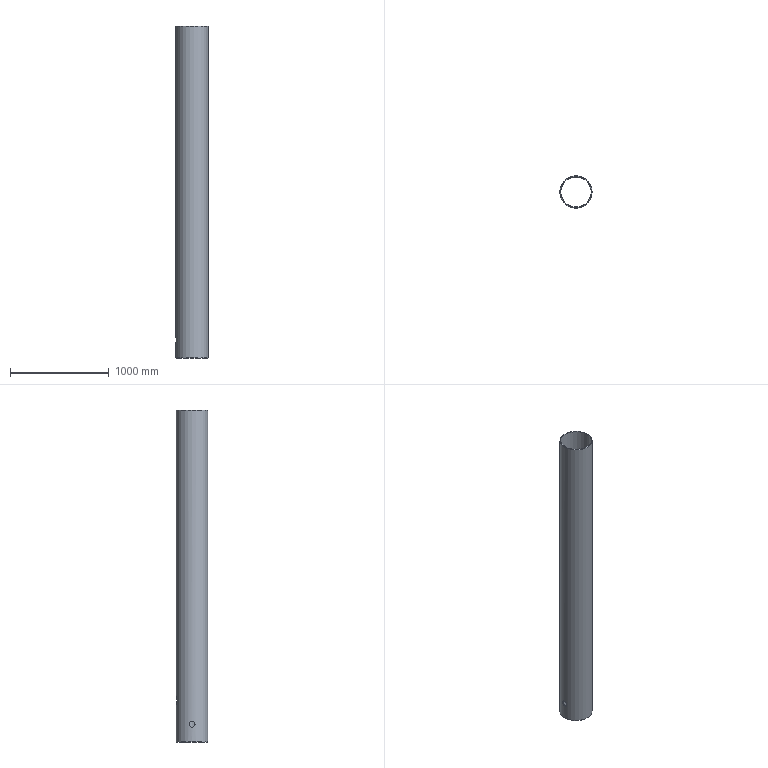Part | NX | features DATUM_CSYS 3, EXTRUDE 2, SKETCH 2, CHAMFER 1, CYLINDER 1, SHELL 1 | 1 solid | 8 faces | box 325 x 325 x 3360 mm | volume 26652772 mm3 | cylinder 4 | plane 2 | cone 2 | commonest cylinder face diameters 60 x1 114 x1 309 x1 325 x1
STEP:
#1=CARTESIAN_POINT('',(-162.5,0.,150.));
#2=VERTEX_POINT('',#1);
#3=CARTESIAN_POINT('',(-162.196,11.848,151.588));
#4=CARTESIAN_POINT('',(-162.651,-0.009709,149.209));
#5=CARTESIAN_POINT('',(-162.198,-11.809,151.576));
#6=CARTESIAN_POINT('',(-161.11,-21.766,158.243));
#7=CARTESIAN_POINT('',(-160.015,-28.424,168.193));
#8=CARTESIAN_POINT('',(-159.553,-30.784,179.98));
#9=CARTESIAN_POINT('',(-160.012,-28.438,191.782));
#10=CARTESIAN_POINT('',(-161.11,-21.767,201.759));
#11=CARTESIAN_POINT('',(-162.199,-11.805,208.427));
#12=CARTESIAN_POINT('',(-162.65,-0.01225,210.784));
#13=CARTESIAN_POINT('',(-162.2,11.782,208.436));
#14=CARTESIAN_POINT('',(-161.114,21.742,201.781));
#15=CARTESIAN_POINT('',(-160.016,28.416,191.833));
#16=CARTESIAN_POINT('',(-159.553,30.787,180.022));
#17=CARTESIAN_POINT('',(-160.013,28.436,168.213));
#18=CARTESIAN_POINT('',(-161.109,21.773,158.254));
#19=CARTESIAN_POINT('',(-162.196,11.848,151.588));
#20=CARTESIAN_POINT('',(-162.651,-0.009709,149.209));
#21=CARTESIAN_POINT('',(-162.198,-11.809,151.576));
#22=B_SPLINE_CURVE_WITH_KNOTS('',3,(#3,#4,#5,#6,#7,#8,#9,#10,#11,#12,#13,#14,#15,#16,#17,#18,#19,#20,#21),.UNSPECIFIED.,.T.,.F.,(1,1,1,1,1,1,1,1,1,1,1,1,1,1,1,1,1,1,1,1,1,1,1),(-0.03524,-0.0235,-0.01175,0.,0.01175,0.0235,0.03524,0.04699,0.05874,0.07049,0.08224,0.09398,0.1057,0.1175,0.1292,0.141,0.1527,0.1645,0.1762,0.188,0.1997,0.2115,0.2232),.UNSPECIFIED.);
#23=EDGE_CURVE('',#2,#2,#22,.T.);
#24=ORIENTED_EDGE('',*,*,#23,.F.);
#25=EDGE_LOOP('',(#24));
#26=FACE_BOUND('',#25,.T.);
#27=CARTESIAN_POINT('',(162.5,0.,3357.5));
#28=VERTEX_POINT('',#27);
#29=CARTESIAN_POINT('',(0.,0.,3357.5));
#30=DIRECTION('',(0.,0.,1.));
#31=DIRECTION('',(1.,0.,0.));
#32=AXIS2_PLACEMENT_3D('',#29,#30,#31);
#33=CIRCLE('',#32,162.5);
#34=EDGE_CURVE('',#28,#28,#33,.F.);
#35=ORIENTED_EDGE('',*,*,#34,.T.);
#36=EDGE_LOOP('',(#35));
#37=FACE_BOUND('',#36,.T.);
#38=CARTESIAN_POINT('',(-162.5,0.,2.5));
#39=VERTEX_POINT('',#38);
#40=CARTESIAN_POINT('',(0.,0.,2.5));
#41=DIRECTION('',(0.,0.,-1.));
#42=DIRECTION('',(-1.,0.,0.));
#43=AXIS2_PLACEMENT_3D('',#40,#41,#42);
#44=CIRCLE('',#43,162.5);
#45=EDGE_CURVE('',#39,#39,#44,.F.);
#46=ORIENTED_EDGE('',*,*,#45,.T.);
#47=EDGE_LOOP('',(#46));
#48=FACE_BOUND('',#47,.T.);
#49=CARTESIAN_POINT('',(0.,162.5,363.));
#50=VERTEX_POINT('',#49);
#51=CARTESIAN_POINT('',(-5.67,162.434,363.189));
#52=CARTESIAN_POINT('',(1.9,162.566,362.813));
#53=CARTESIAN_POINT('',(11.251,162.238,363.741));
#54=CARTESIAN_POINT('',(22.111,161.103,367.065));
#55=CARTESIAN_POINT('',(31.923,159.427,372.341));
#56=CARTESIAN_POINT('',(40.588,157.42,379.464));
#57=CARTESIAN_POINT('',(47.651,155.401,388.066));
#58=CARTESIAN_POINT('',(52.068,153.944,396.293));
#59=CARTESIAN_POINT('',(54.59,153.059,403.281));
#60=CARTESIAN_POINT('',(56.447,152.385,410.637));
#61=CARTESIAN_POINT('',(57.372,152.034,419.919));
#62=CARTESIAN_POINT('',(56.25,152.459,431.302));
#63=CARTESIAN_POINT('',(53.52,153.448,440.229));
#64=CARTESIAN_POINT('',(50.293,154.53,447.019));
#65=CARTESIAN_POINT('',(46.489,155.733,453.343));
#66=CARTESIAN_POINT('',(40.532,157.433,460.588));
#67=CARTESIAN_POINT('',(31.994,159.414,467.612));
#68=CARTESIAN_POINT('',(22.033,161.113,472.966));
#69=CARTESIAN_POINT('',(13.147,162.042,475.687));
#70=CARTESIAN_POINT('',(5.628,162.435,476.816));
#71=CARTESIAN_POINT('',(0.02166,162.532,477.091));
#72=CARTESIAN_POINT('',(-5.585,162.437,476.82));
#73=CARTESIAN_POINT('',(-13.103,162.046,475.698));
#74=CARTESIAN_POINT('',(-22.02,161.115,472.973));
#75=CARTESIAN_POINT('',(-31.981,159.416,467.622));
#76=CARTESIAN_POINT('',(-39.111,157.763,461.756));
#77=CARTESIAN_POINT('',(-44.132,156.407,456.219));
#78=CARTESIAN_POINT('',(-47.426,155.436,451.779));
#79=CARTESIAN_POINT('',(-50.287,154.532,447.032));
#80=CARTESIAN_POINT('',(-53.52,153.448,440.227));
#81=CARTESIAN_POINT('',(-56.238,152.463,431.347));
#82=CARTESIAN_POINT('',(-57.374,152.033,419.959));
#83=CARTESIAN_POINT('',(-56.45,152.384,410.659));
#84=CARTESIAN_POINT('',(-54.598,153.057,403.304));
#85=CARTESIAN_POINT('',(-52.7,153.723,398.047));
#86=CARTESIAN_POINT('',(-50.314,154.523,393.017));
#87=CARTESIAN_POINT('',(-46.44,155.748,386.584));
#88=CARTESIAN_POINT('',(-40.59,157.42,379.468));
#89=CARTESIAN_POINT('',(-31.887,159.434,372.317));
#90=CARTESIAN_POINT('',(-23.755,160.822,367.949));
#91=CARTESIAN_POINT('',(-16.637,161.677,365.384));
#92=CARTESIAN_POINT('',(-11.201,162.144,364.019));
#93=CARTESIAN_POINT('',(-5.67,162.434,363.189));
#94=CARTESIAN_POINT('',(1.9,162.566,362.813));
#95=CARTESIAN_POINT('',(11.251,162.238,363.741));
#96=B_SPLINE_CURVE_WITH_KNOTS('',3,(#51,#52,#53,#54,#55,#56,#57,#58,#59,#60,#61,#62,#63,#64,#65,#66,#67,#68,#69,#70,#71,#72,#73,#74,#75,#76,#77,#78,#79,#80,#81,#82,#83,#84,#85,#86,#87,#88,#89,#90,#91,#92,#93,#94,#95),.UNSPECIFIED.,.T.,.F.,(1,1,1,1,1,1,1,1,1,1,1,1,1,1,1,1,1,1,1,1,1,1,1,1,1,1,1,1,1,1,1,1,1,1,1,1,1,1,1,1,1,1,1,1,1,1,1,1,1),(-0.01684,-0.01123,-0.005613,0.,0.01123,0.02245,0.03368,0.04491,0.05613,0.06736,0.07297,0.07859,0.08981,0.101,0.1123,0.1179,0.1235,0.1347,0.1459,0.1572,0.1684,0.174,0.1796,0.1852,0.1909,0.2021,0.2133,0.2245,0.2301,0.2358,0.2414,0.247,0.2582,0.2694,0.2807,0.2863,0.2919,0.2975,0.3031,0.3143,0.3256,0.3368,0.3424,0.348,0.3536,0.3593,0.3705,0.3817,0.3929),.UNSPECIFIED.);
#97=EDGE_CURVE('',#50,#50,#96,.T.);
#98=ORIENTED_EDGE('',*,*,#97,.T.);
#99=EDGE_LOOP('',(#98));
#100=FACE_BOUND('',#99,.T.);
#101=CARTESIAN_POINT('',(0.,0.,0.));
#102=DIRECTION('',(0.,0.,1.));
#103=DIRECTION('',(1.,0.,0.));
#104=AXIS2_PLACEMENT_3D('',#101,#102,#103);
#105=CYLINDRICAL_SURFACE('',#104,162.5);
#106=ADVANCED_FACE('',(#26,#37,#48,#100),#105,.T.);
#107=CARTESIAN_POINT('',(-154.5,0.,150.));
#108=VERTEX_POINT('',#107);
#109=CARTESIAN_POINT('',(-154.18,11.85,151.589));
#110=CARTESIAN_POINT('',(-154.659,-0.009625,149.209));
#111=CARTESIAN_POINT('',(-154.182,-11.812,151.577));
#112=CARTESIAN_POINT('',(-153.038,-21.766,158.243));
#113=CARTESIAN_POINT('',(-151.884,-28.423,168.19));
#114=CARTESIAN_POINT('',(-151.398,-30.785,179.98));
#115=CARTESIAN_POINT('',(-151.881,-28.437,191.784));
#116=CARTESIAN_POINT('',(-153.038,-21.766,201.76));
#117=CARTESIAN_POINT('',(-154.183,-11.807,208.426));
#118=CARTESIAN_POINT('',(-154.658,-0.01248,210.785));
#119=CARTESIAN_POINT('',(-154.185,11.784,208.435));
#120=CARTESIAN_POINT('',(-153.041,21.742,201.78));
#121=CARTESIAN_POINT('',(-151.886,28.415,191.835));
#122=CARTESIAN_POINT('',(-151.397,30.788,180.021));
#123=CARTESIAN_POINT('',(-151.882,28.435,168.21));
#124=CARTESIAN_POINT('',(-153.036,21.772,158.254));
#125=CARTESIAN_POINT('',(-154.18,11.85,151.589));
#126=CARTESIAN_POINT('',(-154.659,-0.009625,149.209));
#127=CARTESIAN_POINT('',(-154.182,-11.812,151.577));
#128=B_SPLINE_CURVE_WITH_KNOTS('',3,(#109,#110,#111,#112,#113,#114,#115,#116,#117,#118,#119,#120,#121,#122,#123,#124,#125,#126,#127),.UNSPECIFIED.,.T.,.F.,(1,1,1,1,1,1,1,1,1,1,1,1,1,1,1,1,1,1,1,1,1,1,1),(-0.03525,-0.0235,-0.01175,0.,0.01175,0.0235,0.03525,0.047,0.05875,0.0705,0.08225,0.09401,0.1058,0.1175,0.1293,0.141,0.1528,0.1645,0.1763,0.188,0.1998,0.2115,0.2233),.UNSPECIFIED.);
#129=EDGE_CURVE('',#108,#108,#128,.T.);
#130=ORIENTED_EDGE('',*,*,#129,.T.);
#131=EDGE_LOOP('',(#130));
#132=FACE_BOUND('',#131,.T.);
#133=CARTESIAN_POINT('',(154.5,0.,3360.));
#134=VERTEX_POINT('',#133);
#135=CARTESIAN_POINT('',(0.,0.,3360.));
#136=DIRECTION('',(0.,0.,1.));
#137=DIRECTION('',(1.,0.,0.));
#138=AXIS2_PLACEMENT_3D('',#135,#136,#137);
#139=CIRCLE('',#138,154.5);
#140=EDGE_CURVE('',#134,#134,#139,.F.);
#141=ORIENTED_EDGE('',*,*,#140,.F.);
#142=EDGE_LOOP('',(#141));
#143=FACE_BOUND('',#142,.T.);
#144=CARTESIAN_POINT('',(-154.5,0.,0.));
#145=VERTEX_POINT('',#144);
#146=CARTESIAN_POINT('',(0.,0.,0.));
#147=DIRECTION('',(0.,0.,-1.));
#148=DIRECTION('',(-1.,0.,0.));
#149=AXIS2_PLACEMENT_3D('',#146,#147,#148);
#150=CIRCLE('',#149,154.5);
#151=EDGE_CURVE('',#145,#145,#150,.F.);
#152=ORIENTED_EDGE('',*,*,#151,.F.);
#153=EDGE_LOOP('',(#152));
#154=FACE_BOUND('',#153,.T.);
#155=CARTESIAN_POINT('',(0.,154.5,363.));
#156=VERTEX_POINT('',#155);
#157=CARTESIAN_POINT('',(-5.673,154.43,363.19));
#158=CARTESIAN_POINT('',(-0.0003286,154.535,362.905));
#159=CARTESIAN_POINT('',(5.674,154.43,363.19));
#160=CARTESIAN_POINT('',(13.055,154.025,364.294));
#161=CARTESIAN_POINT('',(22.131,153.028,367.071));
#162=CARTESIAN_POINT('',(31.933,151.262,372.35));
#163=CARTESIAN_POINT('',(40.589,149.148,379.466));
#164=CARTESIAN_POINT('',(47.65,147.016,388.065));
#165=CARTESIAN_POINT('',(52.062,145.477,396.281));
#166=CARTESIAN_POINT('',(54.587,144.539,403.271));
#167=CARTESIAN_POINT('',(56.446,143.824,410.63));
#168=CARTESIAN_POINT('',(57.372,143.452,419.92));
#169=CARTESIAN_POINT('',(56.253,143.901,431.303));
#170=CARTESIAN_POINT('',(52.952,145.166,442.06));
#171=CARTESIAN_POINT('',(47.661,147.014,451.928));
#172=CARTESIAN_POINT('',(40.535,149.161,460.582));
#173=CARTESIAN_POINT('',(31.998,151.25,467.61));
#174=CARTESIAN_POINT('',(22.047,153.038,472.961));
#175=CARTESIAN_POINT('',(13.152,154.018,475.687));
#176=CARTESIAN_POINT('',(5.628,154.432,476.816));
#177=CARTESIAN_POINT('',(0.0208,154.534,477.091));
#178=CARTESIAN_POINT('',(-5.595,154.433,476.82));
#179=CARTESIAN_POINT('',(-13.121,154.021,475.694));
#180=CARTESIAN_POINT('',(-22.04,153.04,472.965));
#181=CARTESIAN_POINT('',(-31.993,151.251,467.615));
#182=CARTESIAN_POINT('',(-39.126,149.506,461.741));
#183=CARTESIAN_POINT('',(-44.134,148.078,456.215));
#184=CARTESIAN_POINT('',(-47.425,147.053,451.78));
#185=CARTESIAN_POINT('',(-50.288,146.096,447.031));
#186=CARTESIAN_POINT('',(-53.52,144.949,440.226));
#187=CARTESIAN_POINT('',(-56.237,143.907,431.353));
#188=CARTESIAN_POINT('',(-57.375,143.45,419.95));
#189=CARTESIAN_POINT('',(-56.447,143.823,410.638));
#190=CARTESIAN_POINT('',(-54.591,144.538,403.28));
#191=CARTESIAN_POINT('',(-52.693,145.243,398.029));
#192=CARTESIAN_POINT('',(-50.301,146.091,392.994));
#193=CARTESIAN_POINT('',(-46.426,147.387,386.566));
#194=CARTESIAN_POINT('',(-40.58,149.151,379.459));
#195=CARTESIAN_POINT('',(-31.886,151.273,372.317));
#196=CARTESIAN_POINT('',(-23.749,152.735,367.946));
#197=CARTESIAN_POINT('',(-16.628,153.635,365.381));
#198=CARTESIAN_POINT('',(-11.205,154.126,364.02));
#199=CARTESIAN_POINT('',(-5.673,154.43,363.19));
#200=CARTESIAN_POINT('',(-0.0003286,154.535,362.905));
#201=CARTESIAN_POINT('',(5.674,154.43,363.19));
#202=B_SPLINE_CURVE_WITH_KNOTS('',3,(#157,#158,#159,#160,#161,#162,#163,#164,#165,#166,#167,#168,#169,#170,#171,#172,#173,#174,#175,#176,#177,#178,#179,#180,#181,#182,#183,#184,#185,#186,#187,#188,#189,#190,#191,#192,#193,#194,#195,#196,#197,#198,#199,#200,#201),.UNSPECIFIED.,.T.,.F.,(1,1,1,1,1,1,1,1,1,1,1,1,1,1,1,1,1,1,1,1,1,1,1,1,1,1,1,1,1,1,1,1,1,1,1,1,1,1,1,1,1,1,1,1,1,1,1,1,1),(-0.01686,-0.01124,-0.005618,0.,0.005618,0.01124,0.02247,0.03371,0.04495,0.05618,0.06742,0.07304,0.07866,0.0899,0.1011,0.1124,0.1236,0.1348,0.1461,0.1573,0.1686,0.1742,0.1798,0.1854,0.191,0.2023,0.2135,0.2247,0.2304,0.236,0.2416,0.2472,0.2585,0.2697,0.2809,0.2865,0.2922,0.2978,0.3034,0.3146,0.3259,0.3371,0.3427,0.3483,0.354,0.3596,0.3652,0.3708,0.3821),.UNSPECIFIED.);
#203=EDGE_CURVE('',#156,#156,#202,.T.);
#204=ORIENTED_EDGE('',*,*,#203,.F.);
#205=EDGE_LOOP('',(#204));
#206=FACE_BOUND('',#205,.T.);
#207=CARTESIAN_POINT('',(0.,0.,0.));
#208=DIRECTION('',(0.,0.,1.));
#209=DIRECTION('',(1.,0.,0.));
#210=AXIS2_PLACEMENT_3D('',#207,#208,#209);
#211=CYLINDRICAL_SURFACE('',#210,154.5);
#212=ADVANCED_FACE('',(#132,#143,#154,#206),#211,.F.);
#213=CARTESIAN_POINT('',(158.17,0.,3360.));
#214=VERTEX_POINT('',#213);
#215=CARTESIAN_POINT('',(0.,0.,3360.));
#216=DIRECTION('',(0.,0.,1.));
#217=DIRECTION('',(1.,0.,0.));
#218=AXIS2_PLACEMENT_3D('',#215,#216,#217);
#219=CIRCLE('',#218,158.17);
#220=EDGE_CURVE('',#214,#214,#219,.T.);
#221=ORIENTED_EDGE('',*,*,#220,.T.);
#222=EDGE_LOOP('',(#221));
#223=FACE_BOUND('',#222,.T.);
#224=ORIENTED_EDGE('',*,*,#140,.T.);
#225=EDGE_LOOP('',(#224));
#226=FACE_BOUND('',#225,.T.);
#227=CARTESIAN_POINT('',(0.,0.,3360.));
#228=DIRECTION('',(0.,0.,1.));
#229=DIRECTION('',(1.,0.,0.));
#230=AXIS2_PLACEMENT_3D('',#227,#228,#229);
#231=PLANE('',#230);
#232=ADVANCED_FACE('',(#223,#226),#231,.T.);
#233=CARTESIAN_POINT('',(-158.17,0.,0.));
#234=VERTEX_POINT('',#233);
#235=CARTESIAN_POINT('',(0.,0.,0.));
#236=DIRECTION('',(0.,0.,-1.));
#237=DIRECTION('',(-1.,0.,0.));
#238=AXIS2_PLACEMENT_3D('',#235,#236,#237);
#239=CIRCLE('',#238,158.17);
#240=EDGE_CURVE('',#234,#234,#239,.T.);
#241=ORIENTED_EDGE('',*,*,#240,.T.);
#242=EDGE_LOOP('',(#241));
#243=FACE_BOUND('',#242,.T.);
#244=ORIENTED_EDGE('',*,*,#151,.T.);
#245=EDGE_LOOP('',(#244));
#246=FACE_BOUND('',#245,.T.);
#247=CARTESIAN_POINT('',(0.,0.,0.));
#248=DIRECTION('',(0.,0.,-1.));
#249=DIRECTION('',(-1.,0.,0.));
#250=AXIS2_PLACEMENT_3D('',#247,#248,#249);
#251=PLANE('',#250);
#252=ADVANCED_FACE('',(#243,#246),#251,.T.);
#253=ORIENTED_EDGE('',*,*,#240,.F.);
#254=EDGE_LOOP('',(#253));
#255=FACE_BOUND('',#254,.T.);
#256=ORIENTED_EDGE('',*,*,#45,.F.);
#257=EDGE_LOOP('',(#256));
#258=FACE_BOUND('',#257,.T.);
#259=CARTESIAN_POINT('',(0.,0.,2.5));
#260=DIRECTION('',(0.,0.,1.));
#261=DIRECTION('',(1.,0.,0.));
#262=AXIS2_PLACEMENT_3D('',#259,#260,#261);
#263=CONICAL_SURFACE('',#262,162.5,1.047);
#264=ADVANCED_FACE('',(#255,#258),#263,.T.);
#265=ORIENTED_EDGE('',*,*,#220,.F.);
#266=EDGE_LOOP('',(#265));
#267=FACE_BOUND('',#266,.T.);
#268=ORIENTED_EDGE('',*,*,#34,.F.);
#269=EDGE_LOOP('',(#268));
#270=FACE_BOUND('',#269,.T.);
#271=CARTESIAN_POINT('',(0.,0.,3357.5));
#272=DIRECTION('',(0.,0.,-1.));
#273=DIRECTION('',(-1.,0.,0.));
#274=AXIS2_PLACEMENT_3D('',#271,#272,#273);
#275=CONICAL_SURFACE('',#274,162.5,1.047);
#276=ADVANCED_FACE('',(#267,#270),#275,.T.);
#277=ORIENTED_EDGE('',*,*,#97,.F.);
#278=EDGE_LOOP('',(#277));
#279=FACE_BOUND('',#278,.T.);
#280=ORIENTED_EDGE('',*,*,#203,.T.);
#281=EDGE_LOOP('',(#280));
#282=FACE_BOUND('',#281,.T.);
#283=CARTESIAN_POINT('',(0.,1600.,420.));
#284=DIRECTION('',(0.,-1.,0.));
#285=DIRECTION('',(0.,0.,-1.));
#286=AXIS2_PLACEMENT_3D('',#283,#284,#285);
#287=CYLINDRICAL_SURFACE('',#286,57.);
#288=ADVANCED_FACE('',(#279,#282),#287,.F.);
#289=ORIENTED_EDGE('',*,*,#23,.T.);
#290=EDGE_LOOP('',(#289));
#291=FACE_BOUND('',#290,.T.);
#292=ORIENTED_EDGE('',*,*,#129,.F.);
#293=EDGE_LOOP('',(#292));
#294=FACE_BOUND('',#293,.T.);
#295=CARTESIAN_POINT('',(-670.,0.,180.));
#296=DIRECTION('',(1.,0.,0.));
#297=DIRECTION('',(0.,0.,-1.));
#298=AXIS2_PLACEMENT_3D('',#295,#296,#297);
#299=CYLINDRICAL_SURFACE('',#298,30.);
#300=ADVANCED_FACE('',(#291,#294),#299,.F.);
#301=CLOSED_SHELL('',(#106,#212,#232,#252,#264,#276,#288,#300));
#302=MANIFOLD_SOLID_BREP('',#301);
#303=(LENGTH_UNIT()NAMED_UNIT(*)SI_UNIT(.MILLI.,.METRE.));
#304=UNCERTAINTY_MEASURE_WITH_UNIT(LENGTH_MEASURE(0.0508),#303,'','');
#305=(NAMED_UNIT(*)PLANE_ANGLE_UNIT()SI_UNIT($,.RADIAN.));
#306=(NAMED_UNIT(*)SI_UNIT($,.STERADIAN.)SOLID_ANGLE_UNIT());
#307=(GEOMETRIC_REPRESENTATION_CONTEXT(3)GLOBAL_UNCERTAINTY_ASSIGNED_CONTEXT((#304))GLOBAL_UNIT_ASSIGNED_CONTEXT((#303,#305,#306))REPRESENTATION_CONTEXT('',''));
#308=ADVANCED_BREP_SHAPE_REPRESENTATION('',(#302),#307);